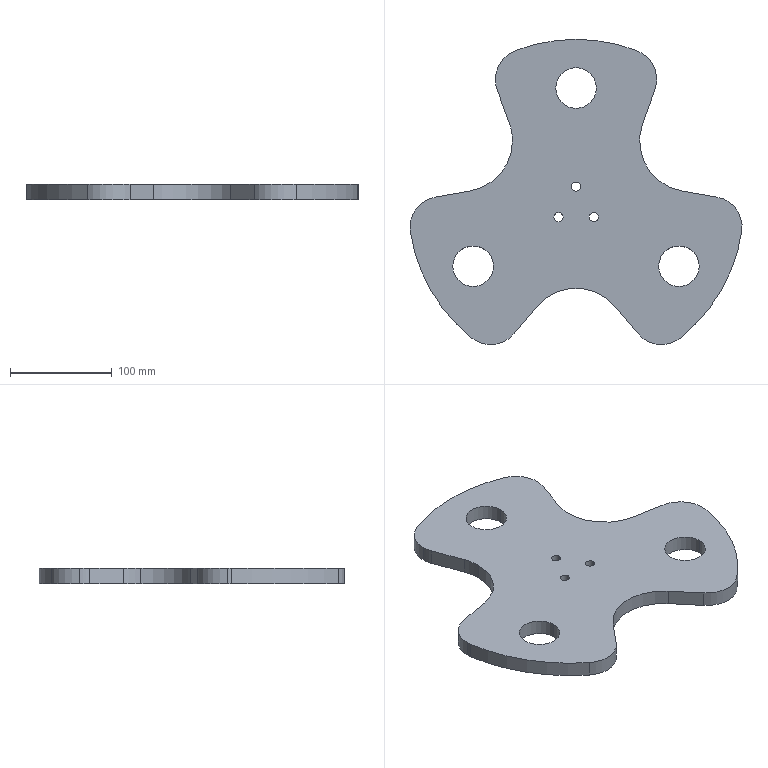Part | SolidWorks | features ICE 2, Extrusion 1, Fillet 1 | 1 solid | 35 faces | box 327.043 x 300.67 x 15 mm | volume 824614 mm3 | cylinder 27 | plane 8 | commonest cylinder face diameters 60 x8 9 x6 40 x6 100 x4 330 x3
STEP:
#1=CARTESIAN_POINT('',(-4.5,20.,0.));
#2=VERTEX_POINT('',#1);
#3=CARTESIAN_POINT('',(4.5,20.,0.));
#4=VERTEX_POINT('',#3);
#5=CARTESIAN_POINT('',(0.,20.,0.));
#6=DIRECTION('',(0.,0.,1.));
#7=DIRECTION('',(1.,0.,0.));
#8=AXIS2_PLACEMENT_3D('',#5,#6,#7);
#9=CIRCLE('',#8,4.5);
#10=EDGE_CURVE('',#2,#4,#9,.T.);
#11=ORIENTED_EDGE('',*,*,#10,.F.);
#12=CARTESIAN_POINT('',(-4.5,20.,15.));
#13=VERTEX_POINT('',#12);
#14=CARTESIAN_POINT('',(-4.5,20.,-5.));
#15=DIRECTION('',(0.,0.,1.));
#16=VECTOR('',#15,1000.);
#17=LINE('',#14,#16);
#18=EDGE_CURVE('',#2,#13,#17,.T.);
#19=ORIENTED_EDGE('',*,*,#18,.T.);
#20=CARTESIAN_POINT('',(4.5,20.,15.));
#21=VERTEX_POINT('',#20);
#22=CARTESIAN_POINT('',(0.,20.,15.));
#23=DIRECTION('',(0.,0.,1.));
#24=DIRECTION('',(1.,0.,0.));
#25=AXIS2_PLACEMENT_3D('',#22,#23,#24);
#26=CIRCLE('',#25,4.5);
#27=EDGE_CURVE('',#13,#21,#26,.T.);
#28=ORIENTED_EDGE('',*,*,#27,.T.);
#29=CARTESIAN_POINT('',(4.5,20.,-5.));
#30=DIRECTION('',(0.,0.,1.));
#31=VECTOR('',#30,1000.);
#32=LINE('',#29,#31);
#33=EDGE_CURVE('',#4,#21,#32,.T.);
#34=ORIENTED_EDGE('',*,*,#33,.F.);
#35=EDGE_LOOP('',(#11,#19,#28,#34));
#36=FACE_OUTER_BOUND('',#35,.T.);
#37=CARTESIAN_POINT('',(0.,20.,-5.));
#38=DIRECTION('',(0.,0.,1.));
#39=DIRECTION('',(1.,0.,0.));
#40=AXIS2_PLACEMENT_3D('',#37,#38,#39);
#41=CYLINDRICAL_SURFACE('',#40,4.5);
#42=ADVANCED_FACE('',(#36),#41,.F.);
#43=CARTESIAN_POINT('',(12.821,-10.,0.));
#44=VERTEX_POINT('',#43);
#45=CARTESIAN_POINT('',(21.821,-10.,0.));
#46=VERTEX_POINT('',#45);
#47=CARTESIAN_POINT('',(17.321,-10.,0.));
#48=DIRECTION('',(0.,0.,1.));
#49=DIRECTION('',(1.,0.,0.));
#50=AXIS2_PLACEMENT_3D('',#47,#48,#49);
#51=CIRCLE('',#50,4.5);
#52=EDGE_CURVE('',#44,#46,#51,.T.);
#53=ORIENTED_EDGE('',*,*,#52,.F.);
#54=CARTESIAN_POINT('',(12.821,-10.,15.));
#55=VERTEX_POINT('',#54);
#56=CARTESIAN_POINT('',(12.821,-10.,-5.));
#57=DIRECTION('',(0.,0.,1.));
#58=VECTOR('',#57,1000.);
#59=LINE('',#56,#58);
#60=EDGE_CURVE('',#44,#55,#59,.T.);
#61=ORIENTED_EDGE('',*,*,#60,.T.);
#62=CARTESIAN_POINT('',(21.821,-10.,15.));
#63=VERTEX_POINT('',#62);
#64=CARTESIAN_POINT('',(17.321,-10.,15.));
#65=DIRECTION('',(0.,0.,1.));
#66=DIRECTION('',(1.,0.,0.));
#67=AXIS2_PLACEMENT_3D('',#64,#65,#66);
#68=CIRCLE('',#67,4.5);
#69=EDGE_CURVE('',#55,#63,#68,.T.);
#70=ORIENTED_EDGE('',*,*,#69,.T.);
#71=CARTESIAN_POINT('',(21.821,-10.,-5.));
#72=DIRECTION('',(0.,0.,1.));
#73=VECTOR('',#72,1000.);
#74=LINE('',#71,#73);
#75=EDGE_CURVE('',#46,#63,#74,.T.);
#76=ORIENTED_EDGE('',*,*,#75,.F.);
#77=EDGE_LOOP('',(#53,#61,#70,#76));
#78=FACE_OUTER_BOUND('',#77,.T.);
#79=CARTESIAN_POINT('',(17.321,-10.,-5.));
#80=DIRECTION('',(0.,0.,1.));
#81=DIRECTION('',(1.,0.,0.));
#82=AXIS2_PLACEMENT_3D('',#79,#80,#81);
#83=CYLINDRICAL_SURFACE('',#82,4.5);
#84=ADVANCED_FACE('',(#78),#83,.F.);
#85=CARTESIAN_POINT('',(-21.821,-10.,0.));
#86=VERTEX_POINT('',#85);
#87=CARTESIAN_POINT('',(-12.821,-10.,0.));
#88=VERTEX_POINT('',#87);
#89=CARTESIAN_POINT('',(-17.321,-10.,0.));
#90=DIRECTION('',(0.,0.,1.));
#91=DIRECTION('',(1.,0.,0.));
#92=AXIS2_PLACEMENT_3D('',#89,#90,#91);
#93=CIRCLE('',#92,4.5);
#94=EDGE_CURVE('',#86,#88,#93,.T.);
#95=ORIENTED_EDGE('',*,*,#94,.F.);
#96=CARTESIAN_POINT('',(-21.821,-10.,15.));
#97=VERTEX_POINT('',#96);
#98=CARTESIAN_POINT('',(-21.821,-10.,-5.));
#99=DIRECTION('',(0.,0.,1.));
#100=VECTOR('',#99,1000.);
#101=LINE('',#98,#100);
#102=EDGE_CURVE('',#86,#97,#101,.T.);
#103=ORIENTED_EDGE('',*,*,#102,.T.);
#104=CARTESIAN_POINT('',(-12.821,-10.,15.));
#105=VERTEX_POINT('',#104);
#106=CARTESIAN_POINT('',(-17.321,-10.,15.));
#107=DIRECTION('',(0.,0.,1.));
#108=DIRECTION('',(1.,0.,0.));
#109=AXIS2_PLACEMENT_3D('',#106,#107,#108);
#110=CIRCLE('',#109,4.5);
#111=EDGE_CURVE('',#97,#105,#110,.T.);
#112=ORIENTED_EDGE('',*,*,#111,.T.);
#113=CARTESIAN_POINT('',(-12.821,-10.,-5.));
#114=DIRECTION('',(0.,0.,1.));
#115=VECTOR('',#114,1000.);
#116=LINE('',#113,#115);
#117=EDGE_CURVE('',#88,#105,#116,.T.);
#118=ORIENTED_EDGE('',*,*,#117,.F.);
#119=EDGE_LOOP('',(#95,#103,#112,#118));
#120=FACE_OUTER_BOUND('',#119,.T.);
#121=CARTESIAN_POINT('',(-17.321,-10.,-5.));
#122=DIRECTION('',(0.,0.,1.));
#123=DIRECTION('',(1.,0.,0.));
#124=AXIS2_PLACEMENT_3D('',#121,#122,#123);
#125=CYLINDRICAL_SURFACE('',#124,4.5);
#126=ADVANCED_FACE('',(#120),#125,.F.);
#127=CARTESIAN_POINT('',(-79.504,125.596,15.));
#128=VERTEX_POINT('',#127);
#129=CARTESIAN_POINT('',(-77.695,115.335,15.));
#130=VERTEX_POINT('',#129);
#131=CARTESIAN_POINT('',(-49.504,125.596,15.));
#132=DIRECTION('',(0.,0.,1.));
#133=DIRECTION('',(1.,0.,0.));
#134=AXIS2_PLACEMENT_3D('',#131,#132,#133);
#135=CIRCLE('',#134,30.);
#136=EDGE_CURVE('',#128,#130,#135,.T.);
#137=ORIENTED_EDGE('',*,*,#136,.F.);
#138=CARTESIAN_POINT('',(-79.504,125.596,0.));
#139=VERTEX_POINT('',#138);
#140=CARTESIAN_POINT('',(-79.504,125.596,15.));
#141=DIRECTION('',(0.,0.,-1.));
#142=VECTOR('',#141,1000.);
#143=LINE('',#140,#142);
#144=EDGE_CURVE('',#128,#139,#143,.T.);
#145=ORIENTED_EDGE('',*,*,#144,.T.);
#146=CARTESIAN_POINT('',(-77.695,115.335,0.));
#147=VERTEX_POINT('',#146);
#148=CARTESIAN_POINT('',(-49.504,125.596,0.));
#149=DIRECTION('',(0.,0.,-1.));
#150=DIRECTION('',(1.,0.,0.));
#151=AXIS2_PLACEMENT_3D('',#148,#149,#150);
#152=CIRCLE('',#151,30.);
#153=EDGE_CURVE('',#147,#139,#152,.T.);
#154=ORIENTED_EDGE('',*,*,#153,.F.);
#155=CARTESIAN_POINT('',(-77.695,115.335,-15.));
#156=DIRECTION('',(0.,0.,-1.));
#157=VECTOR('',#156,1000.);
#158=LINE('',#155,#157);
#159=EDGE_CURVE('',#130,#147,#158,.T.);
#160=ORIENTED_EDGE('',*,*,#159,.F.);
#161=EDGE_LOOP('',(#137,#145,#154,#160));
#162=FACE_OUTER_BOUND('',#161,.T.);
#163=CARTESIAN_POINT('',(-49.504,125.596,15.));
#164=DIRECTION('',(0.,0.,-1.));
#165=DIRECTION('',(-1.,0.,0.));
#166=AXIS2_PLACEMENT_3D('',#163,#164,#165);
#167=CYLINDRICAL_SURFACE('',#166,30.);
#168=ADVANCED_FACE('',(#162),#167,.T.);
#169=CARTESIAN_POINT('',(-163.521,-19.926,15.));
#170=VERTEX_POINT('',#169);
#171=CARTESIAN_POINT('',(-163.193,-24.354,15.));
#172=VERTEX_POINT('',#171);
#173=CARTESIAN_POINT('',(-133.521,-19.926,15.));
#174=DIRECTION('',(0.,0.,1.));
#175=DIRECTION('',(1.,0.,0.));
#176=AXIS2_PLACEMENT_3D('',#173,#174,#175);
#177=CIRCLE('',#176,30.);
#178=EDGE_CURVE('',#170,#172,#177,.T.);
#179=ORIENTED_EDGE('',*,*,#178,.F.);
#180=CARTESIAN_POINT('',(-163.521,-19.926,0.));
#181=VERTEX_POINT('',#180);
#182=CARTESIAN_POINT('',(-163.521,-19.926,15.));
#183=DIRECTION('',(0.,0.,-1.));
#184=VECTOR('',#183,1000.);
#185=LINE('',#182,#184);
#186=EDGE_CURVE('',#170,#181,#185,.T.);
#187=ORIENTED_EDGE('',*,*,#186,.T.);
#188=CARTESIAN_POINT('',(-163.193,-24.354,0.));
#189=VERTEX_POINT('',#188);
#190=CARTESIAN_POINT('',(-133.521,-19.926,0.));
#191=DIRECTION('',(0.,0.,-1.));
#192=DIRECTION('',(1.,0.,0.));
#193=AXIS2_PLACEMENT_3D('',#190,#191,#192);
#194=CIRCLE('',#193,30.);
#195=EDGE_CURVE('',#189,#181,#194,.T.);
#196=ORIENTED_EDGE('',*,*,#195,.F.);
#197=CARTESIAN_POINT('',(-163.193,-24.354,15.));
#198=DIRECTION('',(0.,0.,-1.));
#199=VECTOR('',#198,1000.);
#200=LINE('',#197,#199);
#201=EDGE_CURVE('',#172,#189,#200,.T.);
#202=ORIENTED_EDGE('',*,*,#201,.F.);
#203=EDGE_LOOP('',(#179,#187,#196,#202));
#204=FACE_OUTER_BOUND('',#203,.T.);
#205=CARTESIAN_POINT('',(-133.521,-19.926,15.));
#206=DIRECTION('',(0.,0.,-1.));
#207=DIRECTION('',(-1.,0.,0.));
#208=AXIS2_PLACEMENT_3D('',#205,#206,#207);
#209=CYLINDRICAL_SURFACE('',#208,30.);
#210=ADVANCED_FACE('',(#204),#209,.T.);
#211=CARTESIAN_POINT('',(-62.583,65.,0.));
#212=VERTEX_POINT('',#211);
#213=CARTESIAN_POINT('',(-65.599,82.101,0.));
#214=VERTEX_POINT('',#213);
#215=CARTESIAN_POINT('',(-112.583,65.,0.));
#216=DIRECTION('',(0.,0.,1.));
#217=DIRECTION('',(1.,0.,0.));
#218=AXIS2_PLACEMENT_3D('',#215,#216,#217);
#219=CIRCLE('',#218,50.);
#220=EDGE_CURVE('',#212,#214,#219,.T.);
#221=ORIENTED_EDGE('',*,*,#220,.F.);
#222=CARTESIAN_POINT('',(-62.583,65.,15.));
#223=VERTEX_POINT('',#222);
#224=CARTESIAN_POINT('',(-62.583,65.,-15.));
#225=DIRECTION('',(0.,0.,1.));
#226=VECTOR('',#225,1000.);
#227=LINE('',#224,#226);
#228=EDGE_CURVE('',#212,#223,#227,.T.);
#229=ORIENTED_EDGE('',*,*,#228,.T.);
#230=CARTESIAN_POINT('',(-65.599,82.101,15.));
#231=VERTEX_POINT('',#230);
#232=CARTESIAN_POINT('',(-112.583,65.,15.));
#233=DIRECTION('',(0.,0.,1.));
#234=DIRECTION('',(-1.,0.,0.));
#235=AXIS2_PLACEMENT_3D('',#232,#233,#234);
#236=CIRCLE('',#235,50.);
#237=EDGE_CURVE('',#223,#231,#236,.T.);
#238=ORIENTED_EDGE('',*,*,#237,.T.);
#239=CARTESIAN_POINT('',(-65.599,82.101,-15.));
#240=DIRECTION('',(0.,0.,1.));
#241=VECTOR('',#240,1000.);
#242=LINE('',#239,#241);
#243=EDGE_CURVE('',#214,#231,#242,.T.);
#244=ORIENTED_EDGE('',*,*,#243,.F.);
#245=EDGE_LOOP('',(#221,#229,#238,#244));
#246=FACE_OUTER_BOUND('',#245,.T.);
#247=CARTESIAN_POINT('',(-112.583,65.,-15.));
#248=DIRECTION('',(0.,0.,1.));
#249=DIRECTION('',(1.,0.,0.));
#250=AXIS2_PLACEMENT_3D('',#247,#248,#249);
#251=CYLINDRICAL_SURFACE('',#250,50.);
#252=ADVANCED_FACE('',(#246),#251,.F.);
#253=CARTESIAN_POINT('',(-121.325,-58.5,15.));
#254=VERTEX_POINT('',#253);
#255=CARTESIAN_POINT('',(-81.325,-58.5,15.));
#256=VERTEX_POINT('',#255);
#257=CARTESIAN_POINT('',(-101.325,-58.5,15.));
#258=DIRECTION('',(0.,0.,1.));
#259=DIRECTION('',(1.,0.,0.));
#260=AXIS2_PLACEMENT_3D('',#257,#258,#259);
#261=CIRCLE('',#260,20.);
#262=EDGE_CURVE('',#254,#256,#261,.T.);
#263=ORIENTED_EDGE('',*,*,#262,.T.);
#264=CARTESIAN_POINT('',(-81.325,-58.5,0.));
#265=VERTEX_POINT('',#264);
#266=CARTESIAN_POINT('',(-81.325,-58.5,15.));
#267=DIRECTION('',(0.,0.,-1.));
#268=VECTOR('',#267,1000.);
#269=LINE('',#266,#268);
#270=EDGE_CURVE('',#256,#265,#269,.T.);
#271=ORIENTED_EDGE('',*,*,#270,.T.);
#272=CARTESIAN_POINT('',(-121.325,-58.5,0.));
#273=VERTEX_POINT('',#272);
#274=CARTESIAN_POINT('',(-101.325,-58.5,0.));
#275=DIRECTION('',(0.,0.,1.));
#276=DIRECTION('',(1.,0.,0.));
#277=AXIS2_PLACEMENT_3D('',#274,#275,#276);
#278=CIRCLE('',#277,20.);
#279=EDGE_CURVE('',#273,#265,#278,.T.);
#280=ORIENTED_EDGE('',*,*,#279,.F.);
#281=CARTESIAN_POINT('',(-121.325,-58.5,15.));
#282=DIRECTION('',(0.,0.,-1.));
#283=VECTOR('',#282,1000.);
#284=LINE('',#281,#283);
#285=EDGE_CURVE('',#254,#273,#284,.T.);
#286=ORIENTED_EDGE('',*,*,#285,.F.);
#287=EDGE_LOOP('',(#263,#271,#280,#286));
#288=FACE_OUTER_BOUND('',#287,.T.);
#289=CARTESIAN_POINT('',(-101.325,-58.5,15.));
#290=DIRECTION('',(0.,0.,-1.));
#291=DIRECTION('',(-1.,0.,0.));
#292=AXIS2_PLACEMENT_3D('',#289,#290,#291);
#293=CYLINDRICAL_SURFACE('',#292,20.);
#294=ADVANCED_FACE('',(#288),#293,.F.);
#295=CARTESIAN_POINT('',(81.325,-58.5,15.));
#296=VERTEX_POINT('',#295);
#297=CARTESIAN_POINT('',(121.325,-58.5,15.));
#298=VERTEX_POINT('',#297);
#299=CARTESIAN_POINT('',(101.325,-58.5,15.));
#300=DIRECTION('',(0.,0.,1.));
#301=DIRECTION('',(1.,0.,0.));
#302=AXIS2_PLACEMENT_3D('',#299,#300,#301);
#303=CIRCLE('',#302,20.);
#304=EDGE_CURVE('',#296,#298,#303,.T.);
#305=ORIENTED_EDGE('',*,*,#304,.T.);
#306=CARTESIAN_POINT('',(121.325,-58.5,0.));
#307=VERTEX_POINT('',#306);
#308=CARTESIAN_POINT('',(121.325,-58.5,15.));
#309=DIRECTION('',(0.,0.,-1.));
#310=VECTOR('',#309,1000.);
#311=LINE('',#308,#310);
#312=EDGE_CURVE('',#298,#307,#311,.T.);
#313=ORIENTED_EDGE('',*,*,#312,.T.);
#314=CARTESIAN_POINT('',(81.325,-58.5,0.));
#315=VERTEX_POINT('',#314);
#316=CARTESIAN_POINT('',(101.325,-58.5,0.));
#317=DIRECTION('',(0.,0.,1.));
#318=DIRECTION('',(1.,0.,0.));
#319=AXIS2_PLACEMENT_3D('',#316,#317,#318);
#320=CIRCLE('',#319,20.);
#321=EDGE_CURVE('',#315,#307,#320,.T.);
#322=ORIENTED_EDGE('',*,*,#321,.F.);
#323=CARTESIAN_POINT('',(81.325,-58.5,15.));
#324=DIRECTION('',(0.,0.,-1.));
#325=VECTOR('',#324,1000.);
#326=LINE('',#323,#325);
#327=EDGE_CURVE('',#296,#315,#326,.T.);
#328=ORIENTED_EDGE('',*,*,#327,.F.);
#329=EDGE_LOOP('',(#305,#313,#322,#328));
#330=FACE_OUTER_BOUND('',#329,.T.);
#331=CARTESIAN_POINT('',(101.325,-58.5,15.));
#332=DIRECTION('',(0.,0.,-1.));
#333=DIRECTION('',(-1.,0.,0.));
#334=AXIS2_PLACEMENT_3D('',#331,#332,#333);
#335=CYLINDRICAL_SURFACE('',#334,20.);
#336=ADVANCED_FACE('',(#330),#335,.F.);
#337=CARTESIAN_POINT('',(-20.,117.,15.));
#338=VERTEX_POINT('',#337);
#339=CARTESIAN_POINT('',(20.,117.,15.));
#340=VERTEX_POINT('',#339);
#341=CARTESIAN_POINT('',(0.,117.,15.));
#342=DIRECTION('',(0.,0.,1.));
#343=DIRECTION('',(1.,0.,0.));
#344=AXIS2_PLACEMENT_3D('',#341,#342,#343);
#345=CIRCLE('',#344,20.);
#346=EDGE_CURVE('',#338,#340,#345,.T.);
#347=ORIENTED_EDGE('',*,*,#346,.T.);
#348=CARTESIAN_POINT('',(20.,117.,0.));
#349=VERTEX_POINT('',#348);
#350=CARTESIAN_POINT('',(20.,117.,15.));
#351=DIRECTION('',(0.,0.,-1.));
#352=VECTOR('',#351,1000.);
#353=LINE('',#350,#352);
#354=EDGE_CURVE('',#340,#349,#353,.T.);
#355=ORIENTED_EDGE('',*,*,#354,.T.);
#356=CARTESIAN_POINT('',(-20.,117.,0.));
#357=VERTEX_POINT('',#356);
#358=CARTESIAN_POINT('',(0.,117.,0.));
#359=DIRECTION('',(0.,0.,1.));
#360=DIRECTION('',(1.,0.,0.));
#361=AXIS2_PLACEMENT_3D('',#358,#359,#360);
#362=CIRCLE('',#361,20.);
#363=EDGE_CURVE('',#357,#349,#362,.T.);
#364=ORIENTED_EDGE('',*,*,#363,.F.);
#365=CARTESIAN_POINT('',(-20.,117.,15.));
#366=DIRECTION('',(0.,0.,-1.));
#367=VECTOR('',#366,1000.);
#368=LINE('',#365,#367);
#369=EDGE_CURVE('',#338,#357,#368,.T.);
#370=ORIENTED_EDGE('',*,*,#369,.F.);
#371=EDGE_LOOP('',(#347,#355,#364,#370));
#372=FACE_OUTER_BOUND('',#371,.T.);
#373=CARTESIAN_POINT('',(0.,117.,15.));
#374=DIRECTION('',(0.,0.,-1.));
#375=DIRECTION('',(-1.,0.,0.));
#376=AXIS2_PLACEMENT_3D('',#373,#374,#375);
#377=CYLINDRICAL_SURFACE('',#376,20.);
#378=ADVANCED_FACE('',(#372),#377,.F.);
#379=CARTESIAN_POINT('',(102.688,-129.152,15.));
#380=VERTEX_POINT('',#379);
#381=CARTESIAN_POINT('',(163.193,-24.354,15.));
#382=VERTEX_POINT('',#381);
#383=CARTESIAN_POINT('',(0.,0.,15.));
#384=DIRECTION('',(0.,0.,1.));
#385=DIRECTION('',(1.,0.,0.));
#386=AXIS2_PLACEMENT_3D('',#383,#384,#385);
#387=CIRCLE('',#386,165.);
#388=EDGE_CURVE('',#380,#382,#387,.T.);
#389=ORIENTED_EDGE('',*,*,#388,.F.);
#390=CARTESIAN_POINT('',(102.688,-129.152,0.));
#391=VERTEX_POINT('',#390);
#392=CARTESIAN_POINT('',(102.688,-129.152,15.));
#393=DIRECTION('',(0.,0.,-1.));
#394=VECTOR('',#393,1000.);
#395=LINE('',#392,#394);
#396=EDGE_CURVE('',#380,#391,#395,.T.);
#397=ORIENTED_EDGE('',*,*,#396,.T.);
#398=CARTESIAN_POINT('',(163.193,-24.354,0.));
#399=VERTEX_POINT('',#398);
#400=CARTESIAN_POINT('',(0.,0.,0.));
#401=DIRECTION('',(0.,0.,1.));
#402=DIRECTION('',(1.,0.,0.));
#403=AXIS2_PLACEMENT_3D('',#400,#401,#402);
#404=CIRCLE('',#403,165.);
#405=EDGE_CURVE('',#391,#399,#404,.T.);
#406=ORIENTED_EDGE('',*,*,#405,.T.);
#407=CARTESIAN_POINT('',(163.193,-24.354,15.));
#408=DIRECTION('',(0.,0.,1.));
#409=VECTOR('',#408,1000.);
#410=LINE('',#407,#409);
#411=EDGE_CURVE('',#399,#382,#410,.T.);
#412=ORIENTED_EDGE('',*,*,#411,.T.);
#413=EDGE_LOOP('',(#389,#397,#406,#412));
#414=FACE_OUTER_BOUND('',#413,.T.);
#415=CARTESIAN_POINT('',(0.,0.,15.));
#416=DIRECTION('',(0.,0.,-1.));
#417=DIRECTION('',(-1.,0.,0.));
#418=AXIS2_PLACEMENT_3D('',#415,#416,#417);
#419=CYLINDRICAL_SURFACE('',#418,165.);
#420=ADVANCED_FACE('',(#414),#419,.T.);
#421=CARTESIAN_POINT('',(-102.688,-129.152,0.));
#422=VERTEX_POINT('',#421);
#423=CARTESIAN_POINT('',(0.,0.,0.));
#424=DIRECTION('',(0.,0.,1.));
#425=DIRECTION('',(1.,0.,0.));
#426=AXIS2_PLACEMENT_3D('',#423,#424,#425);
#427=CIRCLE('',#426,165.);
#428=EDGE_CURVE('',#189,#422,#427,.T.);
#429=ORIENTED_EDGE('',*,*,#428,.T.);
#430=CARTESIAN_POINT('',(-102.688,-129.152,15.));
#431=VERTEX_POINT('',#430);
#432=CARTESIAN_POINT('',(-102.688,-129.152,15.));
#433=DIRECTION('',(0.,0.,1.));
#434=VECTOR('',#433,1000.);
#435=LINE('',#432,#434);
#436=EDGE_CURVE('',#422,#431,#435,.T.);
#437=ORIENTED_EDGE('',*,*,#436,.T.);
#438=CARTESIAN_POINT('',(0.,0.,15.));
#439=DIRECTION('',(0.,0.,1.));
#440=DIRECTION('',(1.,0.,0.));
#441=AXIS2_PLACEMENT_3D('',#438,#439,#440);
#442=CIRCLE('',#441,165.);
#443=EDGE_CURVE('',#172,#431,#442,.T.);
#444=ORIENTED_EDGE('',*,*,#443,.F.);
#445=ORIENTED_EDGE('',*,*,#201,.T.);
#446=EDGE_LOOP('',(#429,#437,#444,#445));
#447=FACE_OUTER_BOUND('',#446,.T.);
#448=CARTESIAN_POINT('',(0.,0.,15.));
#449=DIRECTION('',(0.,0.,-1.));
#450=DIRECTION('',(-1.,0.,0.));
#451=AXIS2_PLACEMENT_3D('',#448,#449,#450);
#452=CYLINDRICAL_SURFACE('',#451,165.);
#453=ADVANCED_FACE('',(#447),#452,.T.);
#454=CARTESIAN_POINT('',(0.,20.,15.));
#455=DIRECTION('',(0.,0.,1.));
#456=DIRECTION('',(1.,0.,0.));
#457=AXIS2_PLACEMENT_3D('',#454,#455,#456);
#458=CIRCLE('',#457,4.5);
#459=EDGE_CURVE('',#21,#13,#458,.T.);
#460=ORIENTED_EDGE('',*,*,#459,.F.);
#461=ORIENTED_EDGE('',*,*,#27,.F.);
#462=EDGE_LOOP('',(#460,#461));
#463=FACE_BOUND('',#462,.T.);
#464=CARTESIAN_POINT('',(17.321,-10.,15.));
#465=DIRECTION('',(0.,0.,1.));
#466=DIRECTION('',(1.,0.,0.));
#467=AXIS2_PLACEMENT_3D('',#464,#465,#466);
#468=CIRCLE('',#467,4.5);
#469=EDGE_CURVE('',#63,#55,#468,.T.);
#470=ORIENTED_EDGE('',*,*,#469,.F.);
#471=ORIENTED_EDGE('',*,*,#69,.F.);
#472=EDGE_LOOP('',(#470,#471));
#473=FACE_BOUND('',#472,.T.);
#474=CARTESIAN_POINT('',(-17.321,-10.,15.));
#475=DIRECTION('',(0.,0.,1.));
#476=DIRECTION('',(1.,0.,0.));
#477=AXIS2_PLACEMENT_3D('',#474,#475,#476);
#478=CIRCLE('',#477,4.5);
#479=EDGE_CURVE('',#105,#97,#478,.T.);
#480=ORIENTED_EDGE('',*,*,#479,.F.);
#481=ORIENTED_EDGE('',*,*,#111,.F.);
#482=EDGE_LOOP('',(#480,#481));
#483=FACE_BOUND('',#482,.T.);
#484=ORIENTED_EDGE('',*,*,#443,.T.);
#485=CARTESIAN_POINT('',(-61.036,-124.953,15.));
#486=VERTEX_POINT('',#485);
#487=CARTESIAN_POINT('',(-84.017,-105.67,15.));
#488=DIRECTION('',(0.,0.,1.));
#489=DIRECTION('',(1.,0.,0.));
#490=AXIS2_PLACEMENT_3D('',#487,#488,#489);
#491=CIRCLE('',#490,30.);
#492=EDGE_CURVE('',#431,#486,#491,.T.);
#493=ORIENTED_EDGE('',*,*,#492,.T.);
#494=CARTESIAN_POINT('',(-38.302,-97.861,15.));
#495=VERTEX_POINT('',#494);
#496=CARTESIAN_POINT('',(-38.302,-97.861,15.));
#497=DIRECTION('',(-0.6428,-0.766,0.));
#498=VECTOR('',#497,1000.);
#499=LINE('',#496,#498);
#500=EDGE_CURVE('',#495,#486,#499,.T.);
#501=ORIENTED_EDGE('',*,*,#500,.F.);
#502=CARTESIAN_POINT('',(38.302,-97.861,15.));
#503=VERTEX_POINT('',#502);
#504=CARTESIAN_POINT('',(0.,-130.,15.));
#505=DIRECTION('',(0.,0.,1.));
#506=DIRECTION('',(-1.,0.,0.));
#507=AXIS2_PLACEMENT_3D('',#504,#505,#506);
#508=CIRCLE('',#507,50.);
#509=EDGE_CURVE('',#503,#495,#508,.T.);
#510=ORIENTED_EDGE('',*,*,#509,.F.);
#511=CARTESIAN_POINT('',(61.036,-124.953,15.));
#512=VERTEX_POINT('',#511);
#513=CARTESIAN_POINT('',(115.89,-190.326,15.));
#514=DIRECTION('',(-0.6428,0.766,0.));
#515=VECTOR('',#514,1000.);
#516=LINE('',#513,#515);
#517=EDGE_CURVE('',#512,#503,#516,.T.);
#518=ORIENTED_EDGE('',*,*,#517,.F.);
#519=CARTESIAN_POINT('',(84.017,-105.67,15.));
#520=DIRECTION('',(0.,0.,1.));
#521=DIRECTION('',(1.,0.,0.));
#522=AXIS2_PLACEMENT_3D('',#519,#520,#521);
#523=CIRCLE('',#522,30.);
#524=EDGE_CURVE('',#512,#380,#523,.T.);
#525=ORIENTED_EDGE('',*,*,#524,.T.);
#526=ORIENTED_EDGE('',*,*,#388,.T.);
#527=CARTESIAN_POINT('',(138.731,9.618,15.));
#528=VERTEX_POINT('',#527);
#529=CARTESIAN_POINT('',(133.521,-19.926,15.));
#530=DIRECTION('',(0.,0.,1.));
#531=DIRECTION('',(1.,0.,0.));
#532=AXIS2_PLACEMENT_3D('',#529,#530,#531);
#533=CIRCLE('',#532,30.);
#534=EDGE_CURVE('',#382,#528,#533,.T.);
#535=ORIENTED_EDGE('',*,*,#534,.T.);
#536=CARTESIAN_POINT('',(103.901,15.76,15.));
#537=VERTEX_POINT('',#536);
#538=CARTESIAN_POINT('',(103.901,15.76,15.));
#539=DIRECTION('',(0.9848,-0.1736,0.));
#540=VECTOR('',#539,1000.);
#541=LINE('',#538,#540);
#542=EDGE_CURVE('',#537,#528,#541,.T.);
#543=ORIENTED_EDGE('',*,*,#542,.F.);
#544=CARTESIAN_POINT('',(65.599,82.101,15.));
#545=VERTEX_POINT('',#544);
#546=CARTESIAN_POINT('',(112.583,65.,15.));
#547=DIRECTION('',(0.,0.,1.));
#548=DIRECTION('',(-1.,0.,0.));
#549=AXIS2_PLACEMENT_3D('',#546,#547,#548);
#550=CIRCLE('',#549,50.);
#551=EDGE_CURVE('',#545,#537,#550,.T.);
#552=ORIENTED_EDGE('',*,*,#551,.F.);
#553=CARTESIAN_POINT('',(77.695,115.335,15.));
#554=VERTEX_POINT('',#553);
#555=CARTESIAN_POINT('',(106.882,195.527,15.));
#556=DIRECTION('',(-0.342,-0.9397,0.));
#557=VECTOR('',#556,1000.);
#558=LINE('',#555,#557);
#559=EDGE_CURVE('',#554,#545,#558,.T.);
#560=ORIENTED_EDGE('',*,*,#559,.F.);
#561=CARTESIAN_POINT('',(60.505,153.506,15.));
#562=VERTEX_POINT('',#561);
#563=CARTESIAN_POINT('',(49.504,125.596,15.));
#564=DIRECTION('',(0.,0.,1.));
#565=DIRECTION('',(1.,0.,0.));
#566=AXIS2_PLACEMENT_3D('',#563,#564,#565);
#567=CIRCLE('',#566,30.);
#568=EDGE_CURVE('',#554,#562,#567,.T.);
#569=ORIENTED_EDGE('',*,*,#568,.T.);
#570=CARTESIAN_POINT('',(-60.505,153.506,15.));
#571=VERTEX_POINT('',#570);
#572=CARTESIAN_POINT('',(0.,0.,15.));
#573=DIRECTION('',(0.,0.,1.));
#574=DIRECTION('',(1.,0.,0.));
#575=AXIS2_PLACEMENT_3D('',#572,#573,#574);
#576=CIRCLE('',#575,165.);
#577=EDGE_CURVE('',#562,#571,#576,.T.);
#578=ORIENTED_EDGE('',*,*,#577,.T.);
#579=CARTESIAN_POINT('',(-49.504,125.596,15.));
#580=DIRECTION('',(0.,0.,1.));
#581=DIRECTION('',(1.,0.,0.));
#582=AXIS2_PLACEMENT_3D('',#579,#580,#581);
#583=CIRCLE('',#582,30.);
#584=EDGE_CURVE('',#571,#128,#583,.T.);
#585=ORIENTED_EDGE('',*,*,#584,.T.);
#586=ORIENTED_EDGE('',*,*,#136,.T.);
#587=CARTESIAN_POINT('',(-65.599,82.101,15.));
#588=DIRECTION('',(-0.342,0.9397,0.));
#589=VECTOR('',#588,1000.);
#590=LINE('',#587,#589);
#591=EDGE_CURVE('',#231,#130,#590,.T.);
#592=ORIENTED_EDGE('',*,*,#591,.F.);
#593=ORIENTED_EDGE('',*,*,#237,.F.);
#594=CARTESIAN_POINT('',(-103.901,15.76,15.));
#595=VERTEX_POINT('',#594);
#596=CARTESIAN_POINT('',(-112.583,65.,15.));
#597=DIRECTION('',(0.,0.,1.));
#598=DIRECTION('',(-1.,0.,0.));
#599=AXIS2_PLACEMENT_3D('',#596,#597,#598);
#600=CIRCLE('',#599,50.);
#601=EDGE_CURVE('',#595,#223,#600,.T.);
#602=ORIENTED_EDGE('',*,*,#601,.F.);
#603=CARTESIAN_POINT('',(-138.731,9.618,15.));
#604=VERTEX_POINT('',#603);
#605=CARTESIAN_POINT('',(-222.772,-5.201,15.));
#606=DIRECTION('',(0.9848,0.1736,0.));
#607=VECTOR('',#606,1000.);
#608=LINE('',#605,#607);
#609=EDGE_CURVE('',#604,#595,#608,.T.);
#610=ORIENTED_EDGE('',*,*,#609,.F.);
#611=CARTESIAN_POINT('',(-133.521,-19.926,15.));
#612=DIRECTION('',(0.,0.,1.));
#613=DIRECTION('',(1.,0.,0.));
#614=AXIS2_PLACEMENT_3D('',#611,#612,#613);
#615=CIRCLE('',#614,30.);
#616=EDGE_CURVE('',#604,#170,#615,.T.);
#617=ORIENTED_EDGE('',*,*,#616,.T.);
#618=ORIENTED_EDGE('',*,*,#178,.T.);
#619=EDGE_LOOP('',(#484,#493,#501,#510,#518,#525,#526,#535,#543,#552,#560,#569,#578,#585,#586,#592,#593,#602,#610,#617,#618));
#620=FACE_OUTER_BOUND('',#619,.T.);
#621=ORIENTED_EDGE('',*,*,#304,.F.);
#622=CARTESIAN_POINT('',(101.325,-58.5,15.));
#623=DIRECTION('',(0.,0.,1.));
#624=DIRECTION('',(1.,0.,0.));
#625=AXIS2_PLACEMENT_3D('',#622,#623,#624);
#626=CIRCLE('',#625,20.);
#627=EDGE_CURVE('',#298,#296,#626,.T.);
#628=ORIENTED_EDGE('',*,*,#627,.F.);
#629=EDGE_LOOP('',(#621,#628));
#630=FACE_BOUND('',#629,.T.);
#631=ORIENTED_EDGE('',*,*,#346,.F.);
#632=CARTESIAN_POINT('',(0.,117.,15.));
#633=DIRECTION('',(0.,0.,1.));
#634=DIRECTION('',(1.,0.,0.));
#635=AXIS2_PLACEMENT_3D('',#632,#633,#634);
#636=CIRCLE('',#635,20.);
#637=EDGE_CURVE('',#340,#338,#636,.T.);
#638=ORIENTED_EDGE('',*,*,#637,.F.);
#639=EDGE_LOOP('',(#631,#638));
#640=FACE_BOUND('',#639,.T.);
#641=ORIENTED_EDGE('',*,*,#262,.F.);
#642=CARTESIAN_POINT('',(-101.325,-58.5,15.));
#643=DIRECTION('',(0.,0.,1.));
#644=DIRECTION('',(1.,0.,0.));
#645=AXIS2_PLACEMENT_3D('',#642,#643,#644);
#646=CIRCLE('',#645,20.);
#647=EDGE_CURVE('',#256,#254,#646,.T.);
#648=ORIENTED_EDGE('',*,*,#647,.F.);
#649=EDGE_LOOP('',(#641,#648));
#650=FACE_BOUND('',#649,.T.);
#651=CARTESIAN_POINT('',(0.,0.,15.));
#652=DIRECTION('',(0.,0.,1.));
#653=DIRECTION('',(1.,0.,0.));
#654=AXIS2_PLACEMENT_3D('',#651,#652,#653);
#655=PLANE('',#654);
#656=ADVANCED_FACE('',(#463,#473,#483,#620,#630,#640,#650),#655,.T.);
#657=CARTESIAN_POINT('',(0.,20.,0.));
#658=DIRECTION('',(0.,0.,1.));
#659=DIRECTION('',(1.,0.,0.));
#660=AXIS2_PLACEMENT_3D('',#657,#658,#659);
#661=CIRCLE('',#660,4.5);
#662=EDGE_CURVE('',#4,#2,#661,.T.);
#663=ORIENTED_EDGE('',*,*,#662,.T.);
#664=ORIENTED_EDGE('',*,*,#10,.T.);
#665=EDGE_LOOP('',(#663,#664));
#666=FACE_BOUND('',#665,.T.);
#667=CARTESIAN_POINT('',(17.321,-10.,0.));
#668=DIRECTION('',(0.,0.,1.));
#669=DIRECTION('',(1.,0.,0.));
#670=AXIS2_PLACEMENT_3D('',#667,#668,#669);
#671=CIRCLE('',#670,4.5);
#672=EDGE_CURVE('',#46,#44,#671,.T.);
#673=ORIENTED_EDGE('',*,*,#672,.T.);
#674=ORIENTED_EDGE('',*,*,#52,.T.);
#675=EDGE_LOOP('',(#673,#674));
#676=FACE_BOUND('',#675,.T.);
#677=CARTESIAN_POINT('',(-17.321,-10.,0.));
#678=DIRECTION('',(0.,0.,1.));
#679=DIRECTION('',(1.,0.,0.));
#680=AXIS2_PLACEMENT_3D('',#677,#678,#679);
#681=CIRCLE('',#680,4.5);
#682=EDGE_CURVE('',#88,#86,#681,.T.);
#683=ORIENTED_EDGE('',*,*,#682,.T.);
#684=ORIENTED_EDGE('',*,*,#94,.T.);
#685=EDGE_LOOP('',(#683,#684));
#686=FACE_BOUND('',#685,.T.);
#687=CARTESIAN_POINT('',(-38.302,-97.861,0.));
#688=VERTEX_POINT('',#687);
#689=CARTESIAN_POINT('',(-61.036,-124.953,0.));
#690=VERTEX_POINT('',#689);
#691=CARTESIAN_POINT('',(25.71,-21.573,0.));
#692=DIRECTION('',(-0.6428,-0.766,0.));
#693=VECTOR('',#692,1000.);
#694=LINE('',#691,#693);
#695=EDGE_CURVE('',#688,#690,#694,.T.);
#696=ORIENTED_EDGE('',*,*,#695,.T.);
#697=CARTESIAN_POINT('',(-84.017,-105.67,0.));
#698=DIRECTION('',(0.,0.,-1.));
#699=DIRECTION('',(1.,0.,0.));
#700=AXIS2_PLACEMENT_3D('',#697,#698,#699);
#701=CIRCLE('',#700,30.);
#702=EDGE_CURVE('',#690,#422,#701,.T.);
#703=ORIENTED_EDGE('',*,*,#702,.T.);
#704=ORIENTED_EDGE('',*,*,#428,.F.);
#705=ORIENTED_EDGE('',*,*,#195,.T.);
#706=CARTESIAN_POINT('',(-138.731,9.618,0.));
#707=VERTEX_POINT('',#706);
#708=CARTESIAN_POINT('',(-133.521,-19.926,0.));
#709=DIRECTION('',(0.,0.,-1.));
#710=DIRECTION('',(1.,0.,0.));
#711=AXIS2_PLACEMENT_3D('',#708,#709,#710);
#712=CIRCLE('',#711,30.);
#713=EDGE_CURVE('',#181,#707,#712,.T.);
#714=ORIENTED_EDGE('',*,*,#713,.T.);
#715=CARTESIAN_POINT('',(-103.901,15.76,0.));
#716=VERTEX_POINT('',#715);
#717=CARTESIAN_POINT('',(-5.828,33.053,0.));
#718=DIRECTION('',(0.9848,0.1736,0.));
#719=VECTOR('',#718,1000.);
#720=LINE('',#717,#719);
#721=EDGE_CURVE('',#707,#716,#720,.T.);
#722=ORIENTED_EDGE('',*,*,#721,.T.);
#723=CARTESIAN_POINT('',(-112.583,65.,0.));
#724=DIRECTION('',(0.,0.,1.));
#725=DIRECTION('',(1.,0.,0.));
#726=AXIS2_PLACEMENT_3D('',#723,#724,#725);
#727=CIRCLE('',#726,50.);
#728=EDGE_CURVE('',#716,#212,#727,.T.);
#729=ORIENTED_EDGE('',*,*,#728,.T.);
#730=ORIENTED_EDGE('',*,*,#220,.T.);
#731=CARTESIAN_POINT('',(-31.538,-11.479,0.));
#732=DIRECTION('',(-0.342,0.9397,0.));
#733=VECTOR('',#732,1000.);
#734=LINE('',#731,#733);
#735=EDGE_CURVE('',#214,#147,#734,.T.);
#736=ORIENTED_EDGE('',*,*,#735,.T.);
#737=ORIENTED_EDGE('',*,*,#153,.T.);
#738=CARTESIAN_POINT('',(-60.505,153.506,0.));
#739=VERTEX_POINT('',#738);
#740=CARTESIAN_POINT('',(-49.504,125.596,0.));
#741=DIRECTION('',(0.,0.,-1.));
#742=DIRECTION('',(1.,0.,0.));
#743=AXIS2_PLACEMENT_3D('',#740,#741,#742);
#744=CIRCLE('',#743,30.);
#745=EDGE_CURVE('',#139,#739,#744,.T.);
#746=ORIENTED_EDGE('',*,*,#745,.T.);
#747=CARTESIAN_POINT('',(60.505,153.506,0.));
#748=VERTEX_POINT('',#747);
#749=CARTESIAN_POINT('',(0.,0.,0.));
#750=DIRECTION('',(0.,0.,1.));
#751=DIRECTION('',(1.,0.,0.));
#752=AXIS2_PLACEMENT_3D('',#749,#750,#751);
#753=CIRCLE('',#752,165.);
#754=EDGE_CURVE('',#748,#739,#753,.T.);
#755=ORIENTED_EDGE('',*,*,#754,.F.);
#756=CARTESIAN_POINT('',(77.695,115.335,0.));
#757=VERTEX_POINT('',#756);
#758=CARTESIAN_POINT('',(49.504,125.596,0.));
#759=DIRECTION('',(0.,0.,-1.));
#760=DIRECTION('',(1.,0.,0.));
#761=AXIS2_PLACEMENT_3D('',#758,#759,#760);
#762=CIRCLE('',#761,30.);
#763=EDGE_CURVE('',#748,#757,#762,.T.);
#764=ORIENTED_EDGE('',*,*,#763,.T.);
#765=CARTESIAN_POINT('',(65.599,82.101,0.));
#766=VERTEX_POINT('',#765);
#767=CARTESIAN_POINT('',(31.538,-11.479,0.));
#768=DIRECTION('',(-0.342,-0.9397,0.));
#769=VECTOR('',#768,1000.);
#770=LINE('',#767,#769);
#771=EDGE_CURVE('',#757,#766,#770,.T.);
#772=ORIENTED_EDGE('',*,*,#771,.T.);
#773=CARTESIAN_POINT('',(103.901,15.76,0.));
#774=VERTEX_POINT('',#773);
#775=CARTESIAN_POINT('',(112.583,65.,0.));
#776=DIRECTION('',(0.,0.,1.));
#777=DIRECTION('',(1.,0.,0.));
#778=AXIS2_PLACEMENT_3D('',#775,#776,#777);
#779=CIRCLE('',#778,50.);
#780=EDGE_CURVE('',#766,#774,#779,.T.);
#781=ORIENTED_EDGE('',*,*,#780,.T.);
#782=CARTESIAN_POINT('',(138.731,9.618,0.));
#783=VERTEX_POINT('',#782);
#784=CARTESIAN_POINT('',(5.828,33.053,0.));
#785=DIRECTION('',(0.9848,-0.1736,0.));
#786=VECTOR('',#785,1000.);
#787=LINE('',#784,#786);
#788=EDGE_CURVE('',#774,#783,#787,.T.);
#789=ORIENTED_EDGE('',*,*,#788,.T.);
#790=CARTESIAN_POINT('',(133.521,-19.926,0.));
#791=DIRECTION('',(0.,0.,-1.));
#792=DIRECTION('',(1.,0.,0.));
#793=AXIS2_PLACEMENT_3D('',#790,#791,#792);
#794=CIRCLE('',#793,30.);
#795=EDGE_CURVE('',#783,#399,#794,.T.);
#796=ORIENTED_EDGE('',*,*,#795,.T.);
#797=ORIENTED_EDGE('',*,*,#405,.F.);
#798=CARTESIAN_POINT('',(61.036,-124.953,0.));
#799=VERTEX_POINT('',#798);
#800=CARTESIAN_POINT('',(84.017,-105.67,0.));
#801=DIRECTION('',(0.,0.,-1.));
#802=DIRECTION('',(1.,0.,0.));
#803=AXIS2_PLACEMENT_3D('',#800,#801,#802);
#804=CIRCLE('',#803,30.);
#805=EDGE_CURVE('',#391,#799,#804,.T.);
#806=ORIENTED_EDGE('',*,*,#805,.T.);
#807=CARTESIAN_POINT('',(38.302,-97.861,0.));
#808=VERTEX_POINT('',#807);
#809=CARTESIAN_POINT('',(-25.71,-21.573,0.));
#810=DIRECTION('',(-0.6428,0.766,0.));
#811=VECTOR('',#810,1000.);
#812=LINE('',#809,#811);
#813=EDGE_CURVE('',#799,#808,#812,.T.);
#814=ORIENTED_EDGE('',*,*,#813,.T.);
#815=CARTESIAN_POINT('',(0.,-130.,0.));
#816=DIRECTION('',(0.,0.,1.));
#817=DIRECTION('',(1.,0.,0.));
#818=AXIS2_PLACEMENT_3D('',#815,#816,#817);
#819=CIRCLE('',#818,50.);
#820=EDGE_CURVE('',#808,#688,#819,.T.);
#821=ORIENTED_EDGE('',*,*,#820,.T.);
#822=EDGE_LOOP('',(#696,#703,#704,#705,#714,#722,#729,#730,#736,#737,#746,#755,#764,#772,#781,#789,#796,#797,#806,#814,#821));
#823=FACE_OUTER_BOUND('',#822,.T.);
#824=ORIENTED_EDGE('',*,*,#363,.T.);
#825=CARTESIAN_POINT('',(0.,117.,0.));
#826=DIRECTION('',(0.,0.,1.));
#827=DIRECTION('',(1.,0.,0.));
#828=AXIS2_PLACEMENT_3D('',#825,#826,#827);
#829=CIRCLE('',#828,20.);
#830=EDGE_CURVE('',#349,#357,#829,.T.);
#831=ORIENTED_EDGE('',*,*,#830,.T.);
#832=EDGE_LOOP('',(#824,#831));
#833=FACE_BOUND('',#832,.T.);
#834=ORIENTED_EDGE('',*,*,#321,.T.);
#835=CARTESIAN_POINT('',(101.325,-58.5,0.));
#836=DIRECTION('',(0.,0.,1.));
#837=DIRECTION('',(1.,0.,0.));
#838=AXIS2_PLACEMENT_3D('',#835,#836,#837);
#839=CIRCLE('',#838,20.);
#840=EDGE_CURVE('',#307,#315,#839,.T.);
#841=ORIENTED_EDGE('',*,*,#840,.T.);
#842=EDGE_LOOP('',(#834,#841));
#843=FACE_BOUND('',#842,.T.);
#844=ORIENTED_EDGE('',*,*,#279,.T.);
#845=CARTESIAN_POINT('',(-101.325,-58.5,0.));
#846=DIRECTION('',(0.,0.,1.));
#847=DIRECTION('',(1.,0.,0.));
#848=AXIS2_PLACEMENT_3D('',#845,#846,#847);
#849=CIRCLE('',#848,20.);
#850=EDGE_CURVE('',#265,#273,#849,.T.);
#851=ORIENTED_EDGE('',*,*,#850,.T.);
#852=EDGE_LOOP('',(#844,#851));
#853=FACE_BOUND('',#852,.T.);
#854=CARTESIAN_POINT('',(0.,0.,0.));
#855=DIRECTION('',(0.,0.,1.));
#856=DIRECTION('',(1.,0.,0.));
#857=AXIS2_PLACEMENT_3D('',#854,#855,#856);
#858=PLANE('',#857);
#859=ADVANCED_FACE('',(#666,#676,#686,#823,#833,#843,#853),#858,.F.);
#860=ORIENTED_EDGE('',*,*,#577,.F.);
#861=CARTESIAN_POINT('',(60.505,153.506,15.));
#862=DIRECTION('',(0.,0.,-1.));
#863=VECTOR('',#862,1000.);
#864=LINE('',#861,#863);
#865=EDGE_CURVE('',#562,#748,#864,.T.);
#866=ORIENTED_EDGE('',*,*,#865,.T.);
#867=ORIENTED_EDGE('',*,*,#754,.T.);
#868=CARTESIAN_POINT('',(-60.505,153.506,15.));
#869=DIRECTION('',(0.,0.,1.));
#870=VECTOR('',#869,1000.);
#871=LINE('',#868,#870);
#872=EDGE_CURVE('',#739,#571,#871,.T.);
#873=ORIENTED_EDGE('',*,*,#872,.T.);
#874=EDGE_LOOP('',(#860,#866,#867,#873));
#875=FACE_OUTER_BOUND('',#874,.T.);
#876=CARTESIAN_POINT('',(0.,0.,15.));
#877=DIRECTION('',(0.,0.,-1.));
#878=DIRECTION('',(-1.,0.,0.));
#879=AXIS2_PLACEMENT_3D('',#876,#877,#878);
#880=CYLINDRICAL_SURFACE('',#879,165.);
#881=ADVANCED_FACE('',(#875),#880,.T.);
#882=ORIENTED_EDGE('',*,*,#354,.F.);
#883=ORIENTED_EDGE('',*,*,#637,.T.);
#884=ORIENTED_EDGE('',*,*,#369,.T.);
#885=ORIENTED_EDGE('',*,*,#830,.F.);
#886=EDGE_LOOP('',(#882,#883,#884,#885));
#887=FACE_OUTER_BOUND('',#886,.T.);
#888=CARTESIAN_POINT('',(0.,117.,15.));
#889=DIRECTION('',(0.,0.,-1.));
#890=DIRECTION('',(-1.,0.,0.));
#891=AXIS2_PLACEMENT_3D('',#888,#889,#890);
#892=CYLINDRICAL_SURFACE('',#891,20.);
#893=ADVANCED_FACE('',(#887),#892,.F.);
#894=ORIENTED_EDGE('',*,*,#312,.F.);
#895=ORIENTED_EDGE('',*,*,#627,.T.);
#896=ORIENTED_EDGE('',*,*,#327,.T.);
#897=ORIENTED_EDGE('',*,*,#840,.F.);
#898=EDGE_LOOP('',(#894,#895,#896,#897));
#899=FACE_OUTER_BOUND('',#898,.T.);
#900=CARTESIAN_POINT('',(101.325,-58.5,15.));
#901=DIRECTION('',(0.,0.,-1.));
#902=DIRECTION('',(-1.,0.,0.));
#903=AXIS2_PLACEMENT_3D('',#900,#901,#902);
#904=CYLINDRICAL_SURFACE('',#903,20.);
#905=ADVANCED_FACE('',(#899),#904,.F.);
#906=ORIENTED_EDGE('',*,*,#270,.F.);
#907=ORIENTED_EDGE('',*,*,#647,.T.);
#908=ORIENTED_EDGE('',*,*,#285,.T.);
#909=ORIENTED_EDGE('',*,*,#850,.F.);
#910=EDGE_LOOP('',(#906,#907,#908,#909));
#911=FACE_OUTER_BOUND('',#910,.T.);
#912=CARTESIAN_POINT('',(-101.325,-58.5,15.));
#913=DIRECTION('',(0.,0.,-1.));
#914=DIRECTION('',(-1.,0.,0.));
#915=AXIS2_PLACEMENT_3D('',#912,#913,#914);
#916=CYLINDRICAL_SURFACE('',#915,20.);
#917=ADVANCED_FACE('',(#911),#916,.F.);
#918=CARTESIAN_POINT('',(65.599,82.101,-15.));
#919=DIRECTION('',(0.,0.,1.));
#920=VECTOR('',#919,1000.);
#921=LINE('',#918,#920);
#922=EDGE_CURVE('',#766,#545,#921,.T.);
#923=ORIENTED_EDGE('',*,*,#922,.T.);
#924=ORIENTED_EDGE('',*,*,#551,.T.);
#925=CARTESIAN_POINT('',(103.901,15.76,-15.));
#926=DIRECTION('',(0.,0.,1.));
#927=VECTOR('',#926,1000.);
#928=LINE('',#925,#927);
#929=EDGE_CURVE('',#774,#537,#928,.T.);
#930=ORIENTED_EDGE('',*,*,#929,.F.);
#931=ORIENTED_EDGE('',*,*,#780,.F.);
#932=EDGE_LOOP('',(#923,#924,#930,#931));
#933=FACE_OUTER_BOUND('',#932,.T.);
#934=CARTESIAN_POINT('',(112.583,65.,-15.));
#935=DIRECTION('',(0.,0.,1.));
#936=DIRECTION('',(1.,0.,0.));
#937=AXIS2_PLACEMENT_3D('',#934,#935,#936);
#938=CYLINDRICAL_SURFACE('',#937,50.);
#939=ADVANCED_FACE('',(#933),#938,.F.);
#940=ORIENTED_EDGE('',*,*,#771,.F.);
#941=CARTESIAN_POINT('',(77.695,115.335,-15.));
#942=DIRECTION('',(0.,0.,1.));
#943=VECTOR('',#942,1000.);
#944=LINE('',#941,#943);
#945=EDGE_CURVE('',#757,#554,#944,.T.);
#946=ORIENTED_EDGE('',*,*,#945,.T.);
#947=ORIENTED_EDGE('',*,*,#559,.T.);
#948=ORIENTED_EDGE('',*,*,#922,.F.);
#949=EDGE_LOOP('',(#940,#946,#947,#948));
#950=FACE_OUTER_BOUND('',#949,.T.);
#951=CARTESIAN_POINT('',(106.882,195.527,-15.));
#952=DIRECTION('',(-0.9397,0.342,0.));
#953=DIRECTION('',(-0.342,-0.9397,0.));
#954=AXIS2_PLACEMENT_3D('',#951,#952,#953);
#955=PLANE('',#954);
#956=ADVANCED_FACE('',(#950),#955,.F.);
#957=ORIENTED_EDGE('',*,*,#542,.T.);
#958=CARTESIAN_POINT('',(138.731,9.618,-15.));
#959=DIRECTION('',(0.,0.,-1.));
#960=VECTOR('',#959,1000.);
#961=LINE('',#958,#960);
#962=EDGE_CURVE('',#528,#783,#961,.T.);
#963=ORIENTED_EDGE('',*,*,#962,.T.);
#964=ORIENTED_EDGE('',*,*,#788,.F.);
#965=ORIENTED_EDGE('',*,*,#929,.T.);
#966=EDGE_LOOP('',(#957,#963,#964,#965));
#967=FACE_OUTER_BOUND('',#966,.T.);
#968=CARTESIAN_POINT('',(103.901,15.76,-15.));
#969=DIRECTION('',(-0.1736,-0.9848,0.));
#970=DIRECTION('',(0.9848,-0.1736,0.));
#971=AXIS2_PLACEMENT_3D('',#968,#969,#970);
#972=PLANE('',#971);
#973=ADVANCED_FACE('',(#967),#972,.F.);
#974=ORIENTED_EDGE('',*,*,#228,.F.);
#975=ORIENTED_EDGE('',*,*,#728,.F.);
#976=CARTESIAN_POINT('',(-103.901,15.76,-15.));
#977=DIRECTION('',(0.,0.,1.));
#978=VECTOR('',#977,1000.);
#979=LINE('',#976,#978);
#980=EDGE_CURVE('',#716,#595,#979,.T.);
#981=ORIENTED_EDGE('',*,*,#980,.T.);
#982=ORIENTED_EDGE('',*,*,#601,.T.);
#983=EDGE_LOOP('',(#974,#975,#981,#982));
#984=FACE_OUTER_BOUND('',#983,.T.);
#985=CARTESIAN_POINT('',(-112.583,65.,-15.));
#986=DIRECTION('',(0.,0.,1.));
#987=DIRECTION('',(1.,0.,0.));
#988=AXIS2_PLACEMENT_3D('',#985,#986,#987);
#989=CYLINDRICAL_SURFACE('',#988,50.);
#990=ADVANCED_FACE('',(#984),#989,.F.);
#991=ORIENTED_EDGE('',*,*,#721,.F.);
#992=CARTESIAN_POINT('',(-138.731,9.618,-15.));
#993=DIRECTION('',(0.,0.,1.));
#994=VECTOR('',#993,1000.);
#995=LINE('',#992,#994);
#996=EDGE_CURVE('',#707,#604,#995,.T.);
#997=ORIENTED_EDGE('',*,*,#996,.T.);
#998=ORIENTED_EDGE('',*,*,#609,.T.);
#999=ORIENTED_EDGE('',*,*,#980,.F.);
#1000=EDGE_LOOP('',(#991,#997,#998,#999));
#1001=FACE_OUTER_BOUND('',#1000,.T.);
#1002=CARTESIAN_POINT('',(-222.772,-5.201,-15.));
#1003=DIRECTION('',(0.1736,-0.9848,0.));
#1004=DIRECTION('',(0.9848,0.1736,0.));
#1005=AXIS2_PLACEMENT_3D('',#1002,#1003,#1004);
#1006=PLANE('',#1005);
#1007=ADVANCED_FACE('',(#1001),#1006,.F.);
#1008=ORIENTED_EDGE('',*,*,#591,.T.);
#1009=ORIENTED_EDGE('',*,*,#159,.T.);
#1010=ORIENTED_EDGE('',*,*,#735,.F.);
#1011=ORIENTED_EDGE('',*,*,#243,.T.);
#1012=EDGE_LOOP('',(#1008,#1009,#1010,#1011));
#1013=FACE_OUTER_BOUND('',#1012,.T.);
#1014=CARTESIAN_POINT('',(-65.599,82.101,-15.));
#1015=DIRECTION('',(0.9397,0.342,0.));
#1016=DIRECTION('',(-0.342,0.9397,0.));
#1017=AXIS2_PLACEMENT_3D('',#1014,#1015,#1016);
#1018=PLANE('',#1017);
#1019=ADVANCED_FACE('',(#1013),#1018,.F.);
#1020=CARTESIAN_POINT('',(38.302,-97.861,-15.));
#1021=DIRECTION('',(0.,0.,1.));
#1022=VECTOR('',#1021,1000.);
#1023=LINE('',#1020,#1022);
#1024=EDGE_CURVE('',#808,#503,#1023,.T.);
#1025=ORIENTED_EDGE('',*,*,#1024,.T.);
#1026=ORIENTED_EDGE('',*,*,#509,.T.);
#1027=CARTESIAN_POINT('',(-38.302,-97.861,-15.));
#1028=DIRECTION('',(0.,0.,1.));
#1029=VECTOR('',#1028,1000.);
#1030=LINE('',#1027,#1029);
#1031=EDGE_CURVE('',#688,#495,#1030,.T.);
#1032=ORIENTED_EDGE('',*,*,#1031,.F.);
#1033=ORIENTED_EDGE('',*,*,#820,.F.);
#1034=EDGE_LOOP('',(#1025,#1026,#1032,#1033));
#1035=FACE_OUTER_BOUND('',#1034,.T.);
#1036=CARTESIAN_POINT('',(0.,-130.,-15.));
#1037=DIRECTION('',(0.,0.,1.));
#1038=DIRECTION('',(1.,0.,0.));
#1039=AXIS2_PLACEMENT_3D('',#1036,#1037,#1038);
#1040=CYLINDRICAL_SURFACE('',#1039,50.);
#1041=ADVANCED_FACE('',(#1035),#1040,.F.);
#1042=ORIENTED_EDGE('',*,*,#813,.F.);
#1043=CARTESIAN_POINT('',(61.036,-124.953,-15.));
#1044=DIRECTION('',(0.,0.,1.));
#1045=VECTOR('',#1044,1000.);
#1046=LINE('',#1043,#1045);
#1047=EDGE_CURVE('',#799,#512,#1046,.T.);
#1048=ORIENTED_EDGE('',*,*,#1047,.T.);
#1049=ORIENTED_EDGE('',*,*,#517,.T.);
#1050=ORIENTED_EDGE('',*,*,#1024,.F.);
#1051=EDGE_LOOP('',(#1042,#1048,#1049,#1050));
#1052=FACE_OUTER_BOUND('',#1051,.T.);
#1053=CARTESIAN_POINT('',(115.89,-190.326,-15.));
#1054=DIRECTION('',(0.766,0.6428,0.));
#1055=DIRECTION('',(-0.6428,0.766,0.));
#1056=AXIS2_PLACEMENT_3D('',#1053,#1054,#1055);
#1057=PLANE('',#1056);
#1058=ADVANCED_FACE('',(#1052),#1057,.F.);
#1059=ORIENTED_EDGE('',*,*,#500,.T.);
#1060=CARTESIAN_POINT('',(-61.036,-124.953,-15.));
#1061=DIRECTION('',(0.,0.,-1.));
#1062=VECTOR('',#1061,1000.);
#1063=LINE('',#1060,#1062);
#1064=EDGE_CURVE('',#486,#690,#1063,.T.);
#1065=ORIENTED_EDGE('',*,*,#1064,.T.);
#1066=ORIENTED_EDGE('',*,*,#695,.F.);
#1067=ORIENTED_EDGE('',*,*,#1031,.T.);
#1068=EDGE_LOOP('',(#1059,#1065,#1066,#1067));
#1069=FACE_OUTER_BOUND('',#1068,.T.);
#1070=CARTESIAN_POINT('',(-38.302,-97.861,-15.));
#1071=DIRECTION('',(-0.766,0.6428,0.));
#1072=DIRECTION('',(-0.6428,-0.766,0.));
#1073=AXIS2_PLACEMENT_3D('',#1070,#1071,#1072);
#1074=PLANE('',#1073);
#1075=ADVANCED_FACE('',(#1069),#1074,.F.);
#1076=ORIENTED_EDGE('',*,*,#702,.F.);
#1077=ORIENTED_EDGE('',*,*,#1064,.F.);
#1078=ORIENTED_EDGE('',*,*,#492,.F.);
#1079=ORIENTED_EDGE('',*,*,#436,.F.);
#1080=EDGE_LOOP('',(#1076,#1077,#1078,#1079));
#1081=FACE_OUTER_BOUND('',#1080,.T.);
#1082=CARTESIAN_POINT('',(-84.017,-105.67,15.));
#1083=DIRECTION('',(0.,0.,-1.));
#1084=DIRECTION('',(-1.,0.,0.));
#1085=AXIS2_PLACEMENT_3D('',#1082,#1083,#1084);
#1086=CYLINDRICAL_SURFACE('',#1085,30.);
#1087=ADVANCED_FACE('',(#1081),#1086,.T.);
#1088=ORIENTED_EDGE('',*,*,#524,.F.);
#1089=ORIENTED_EDGE('',*,*,#1047,.F.);
#1090=ORIENTED_EDGE('',*,*,#805,.F.);
#1091=ORIENTED_EDGE('',*,*,#396,.F.);
#1092=EDGE_LOOP('',(#1088,#1089,#1090,#1091));
#1093=FACE_OUTER_BOUND('',#1092,.T.);
#1094=CARTESIAN_POINT('',(84.017,-105.67,15.));
#1095=DIRECTION('',(0.,0.,-1.));
#1096=DIRECTION('',(-1.,0.,0.));
#1097=AXIS2_PLACEMENT_3D('',#1094,#1095,#1096);
#1098=CYLINDRICAL_SURFACE('',#1097,30.);
#1099=ADVANCED_FACE('',(#1093),#1098,.T.);
#1100=ORIENTED_EDGE('',*,*,#795,.F.);
#1101=ORIENTED_EDGE('',*,*,#962,.F.);
#1102=ORIENTED_EDGE('',*,*,#534,.F.);
#1103=ORIENTED_EDGE('',*,*,#411,.F.);
#1104=EDGE_LOOP('',(#1100,#1101,#1102,#1103));
#1105=FACE_OUTER_BOUND('',#1104,.T.);
#1106=CARTESIAN_POINT('',(133.521,-19.926,15.));
#1107=DIRECTION('',(0.,0.,-1.));
#1108=DIRECTION('',(-1.,0.,0.));
#1109=AXIS2_PLACEMENT_3D('',#1106,#1107,#1108);
#1110=CYLINDRICAL_SURFACE('',#1109,30.);
#1111=ADVANCED_FACE('',(#1105),#1110,.T.);
#1112=ORIENTED_EDGE('',*,*,#568,.F.);
#1113=ORIENTED_EDGE('',*,*,#945,.F.);
#1114=ORIENTED_EDGE('',*,*,#763,.F.);
#1115=ORIENTED_EDGE('',*,*,#865,.F.);
#1116=EDGE_LOOP('',(#1112,#1113,#1114,#1115));
#1117=FACE_OUTER_BOUND('',#1116,.T.);
#1118=CARTESIAN_POINT('',(49.504,125.596,15.));
#1119=DIRECTION('',(0.,0.,-1.));
#1120=DIRECTION('',(-1.,0.,0.));
#1121=AXIS2_PLACEMENT_3D('',#1118,#1119,#1120);
#1122=CYLINDRICAL_SURFACE('',#1121,30.);
#1123=ADVANCED_FACE('',(#1117),#1122,.T.);
#1124=ORIENTED_EDGE('',*,*,#186,.F.);
#1125=ORIENTED_EDGE('',*,*,#616,.F.);
#1126=ORIENTED_EDGE('',*,*,#996,.F.);
#1127=ORIENTED_EDGE('',*,*,#713,.F.);
#1128=EDGE_LOOP('',(#1124,#1125,#1126,#1127));
#1129=FACE_OUTER_BOUND('',#1128,.T.);
#1130=CARTESIAN_POINT('',(-133.521,-19.926,15.));
#1131=DIRECTION('',(0.,0.,-1.));
#1132=DIRECTION('',(-1.,0.,0.));
#1133=AXIS2_PLACEMENT_3D('',#1130,#1131,#1132);
#1134=CYLINDRICAL_SURFACE('',#1133,30.);
#1135=ADVANCED_FACE('',(#1129),#1134,.T.);
#1136=ORIENTED_EDGE('',*,*,#144,.F.);
#1137=ORIENTED_EDGE('',*,*,#584,.F.);
#1138=ORIENTED_EDGE('',*,*,#872,.F.);
#1139=ORIENTED_EDGE('',*,*,#745,.F.);
#1140=EDGE_LOOP('',(#1136,#1137,#1138,#1139));
#1141=FACE_OUTER_BOUND('',#1140,.T.);
#1142=CARTESIAN_POINT('',(-49.504,125.596,15.));
#1143=DIRECTION('',(0.,0.,-1.));
#1144=DIRECTION('',(-1.,0.,0.));
#1145=AXIS2_PLACEMENT_3D('',#1142,#1143,#1144);
#1146=CYLINDRICAL_SURFACE('',#1145,30.);
#1147=ADVANCED_FACE('',(#1141),#1146,.T.);
#1148=ORIENTED_EDGE('',*,*,#102,.F.);
#1149=ORIENTED_EDGE('',*,*,#682,.F.);
#1150=ORIENTED_EDGE('',*,*,#117,.T.);
#1151=ORIENTED_EDGE('',*,*,#479,.T.);
#1152=EDGE_LOOP('',(#1148,#1149,#1150,#1151));
#1153=FACE_OUTER_BOUND('',#1152,.T.);
#1154=CARTESIAN_POINT('',(-17.321,-10.,-5.));
#1155=DIRECTION('',(0.,0.,1.));
#1156=DIRECTION('',(1.,0.,0.));
#1157=AXIS2_PLACEMENT_3D('',#1154,#1155,#1156);
#1158=CYLINDRICAL_SURFACE('',#1157,4.5);
#1159=ADVANCED_FACE('',(#1153),#1158,.F.);
#1160=ORIENTED_EDGE('',*,*,#60,.F.);
#1161=ORIENTED_EDGE('',*,*,#672,.F.);
#1162=ORIENTED_EDGE('',*,*,#75,.T.);
#1163=ORIENTED_EDGE('',*,*,#469,.T.);
#1164=EDGE_LOOP('',(#1160,#1161,#1162,#1163));
#1165=FACE_OUTER_BOUND('',#1164,.T.);
#1166=CARTESIAN_POINT('',(17.321,-10.,-5.));
#1167=DIRECTION('',(0.,0.,1.));
#1168=DIRECTION('',(1.,0.,0.));
#1169=AXIS2_PLACEMENT_3D('',#1166,#1167,#1168);
#1170=CYLINDRICAL_SURFACE('',#1169,4.5);
#1171=ADVANCED_FACE('',(#1165),#1170,.F.);
#1172=ORIENTED_EDGE('',*,*,#18,.F.);
#1173=ORIENTED_EDGE('',*,*,#662,.F.);
#1174=ORIENTED_EDGE('',*,*,#33,.T.);
#1175=ORIENTED_EDGE('',*,*,#459,.T.);
#1176=EDGE_LOOP('',(#1172,#1173,#1174,#1175));
#1177=FACE_OUTER_BOUND('',#1176,.T.);
#1178=CARTESIAN_POINT('',(0.,20.,-5.));
#1179=DIRECTION('',(0.,0.,1.));
#1180=DIRECTION('',(1.,0.,0.));
#1181=AXIS2_PLACEMENT_3D('',#1178,#1179,#1180);
#1182=CYLINDRICAL_SURFACE('',#1181,4.5);
#1183=ADVANCED_FACE('',(#1177),#1182,.F.);
#1184=CLOSED_SHELL('',(#42,#84,#126,#168,#210,#252,#294,#336,#378,#420,#453,#656,#859,#881,#893,#905,#917,#939,#956,#973,#990,#1007,#1019,#1041,#1058,#1075,#1087,#1099,#1111,#1123,#1135,#1147,#1159,#1171,#1183));
#1185=MANIFOLD_SOLID_BREP('',#1184);
#1186=CARTESIAN_POINT('',(0.,0.,0.));
#1187=DIRECTION('',(0.,0.,1.));
#1188=DIRECTION('',(1.,0.,0.));
#1189=AXIS2_PLACEMENT_3D('',#1186,#1187,#1188);
#1190=(LENGTH_UNIT()NAMED_UNIT(*)SI_UNIT(.MILLI.,.METRE.));
#1191=UNCERTAINTY_MEASURE_WITH_UNIT(LENGTH_MEASURE(0.00001),#1190,'','');
#1192=(NAMED_UNIT(*)PLANE_ANGLE_UNIT()SI_UNIT($,.RADIAN.));
#1193=(NAMED_UNIT(*)SI_UNIT($,.STERADIAN.)SOLID_ANGLE_UNIT());
#1194=(GEOMETRIC_REPRESENTATION_CONTEXT(3)GLOBAL_UNCERTAINTY_ASSIGNED_CONTEXT((#1191))GLOBAL_UNIT_ASSIGNED_CONTEXT((#1190,#1192,#1193))REPRESENTATION_CONTEXT('',''));
#1195=ADVANCED_BREP_SHAPE_REPRESENTATION('',(#1185,#1189),#1194);